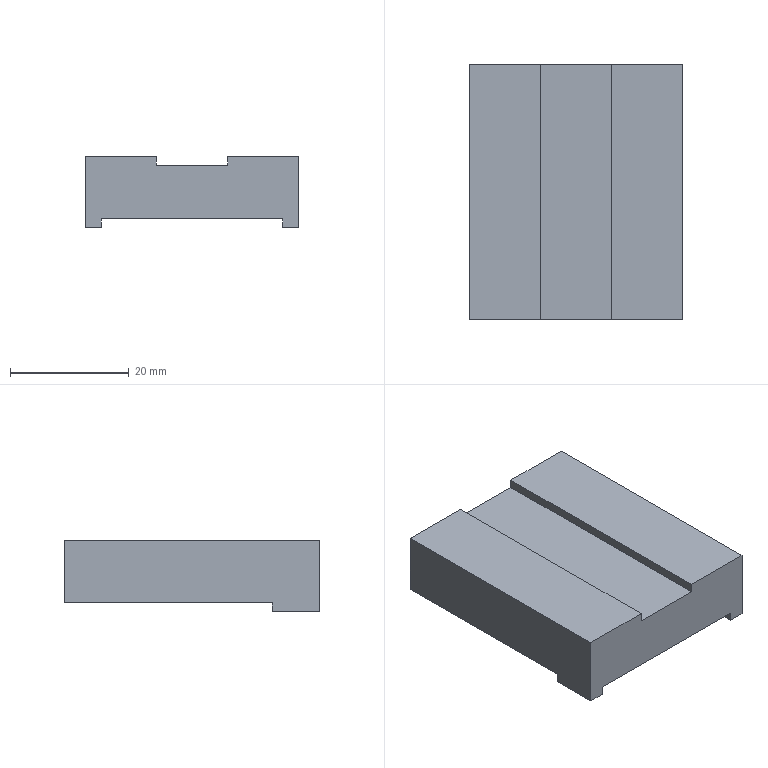Part | SolidWorks | features ICE 3, Extrusion 1 | 1 solid | 16 faces | box 36 x 43 x 12 mm | volume 15546 mm3 | plane 16
STEP:
#1=CARTESIAN_POINT('',(18.,-13.5,-6.));
#2=VERTEX_POINT('',#1);
#3=CARTESIAN_POINT('',(15.25,-13.5,-6.));
#4=VERTEX_POINT('',#3);
#5=CARTESIAN_POINT('',(-18.,-13.5,-6.));
#6=DIRECTION('',(-1.,0.,0.));
#7=VECTOR('',#6,1000.);
#8=LINE('',#5,#7);
#9=EDGE_CURVE('',#2,#4,#8,.T.);
#10=ORIENTED_EDGE('',*,*,#9,.F.);
#11=CARTESIAN_POINT('',(18.,-21.5,-6.));
#12=VERTEX_POINT('',#11);
#13=CARTESIAN_POINT('',(18.,-21.5,-6.));
#14=DIRECTION('',(0.,1.,0.));
#15=VECTOR('',#14,1000.);
#16=LINE('',#13,#15);
#17=EDGE_CURVE('',#12,#2,#16,.T.);
#18=ORIENTED_EDGE('',*,*,#17,.F.);
#19=CARTESIAN_POINT('',(15.25,-21.5,-6.));
#20=VERTEX_POINT('',#19);
#21=CARTESIAN_POINT('',(-18.,-21.5,-6.));
#22=DIRECTION('',(1.,0.,0.));
#23=VECTOR('',#22,1000.);
#24=LINE('',#21,#23);
#25=EDGE_CURVE('',#20,#12,#24,.T.);
#26=ORIENTED_EDGE('',*,*,#25,.F.);
#27=CARTESIAN_POINT('',(15.25,21.5,-6.));
#28=DIRECTION('',(0.,-1.,0.));
#29=VECTOR('',#28,1000.);
#30=LINE('',#27,#29);
#31=EDGE_CURVE('',#4,#20,#30,.T.);
#32=ORIENTED_EDGE('',*,*,#31,.F.);
#33=EDGE_LOOP('',(#10,#18,#26,#32));
#34=FACE_OUTER_BOUND('',#33,.T.);
#35=CARTESIAN_POINT('',(0.,0.,-6.));
#36=DIRECTION('',(0.,0.,-1.));
#37=DIRECTION('',(-1.,0.,0.));
#38=AXIS2_PLACEMENT_3D('',#35,#36,#37);
#39=PLANE('',#38);
#40=ADVANCED_FACE('',(#34),#39,.T.);
#41=CARTESIAN_POINT('',(18.,21.5,6.));
#42=VERTEX_POINT('',#41);
#43=CARTESIAN_POINT('',(6.,21.5,6.));
#44=VERTEX_POINT('',#43);
#45=CARTESIAN_POINT('',(-18.,21.5,6.));
#46=DIRECTION('',(-1.,0.,0.));
#47=VECTOR('',#46,1000.);
#48=LINE('',#45,#47);
#49=EDGE_CURVE('',#42,#44,#48,.T.);
#50=ORIENTED_EDGE('',*,*,#49,.T.);
#51=CARTESIAN_POINT('',(6.,-21.5,6.));
#52=VERTEX_POINT('',#51);
#53=CARTESIAN_POINT('',(6.,21.5,6.));
#54=DIRECTION('',(0.,1.,0.));
#55=VECTOR('',#54,1000.);
#56=LINE('',#53,#55);
#57=EDGE_CURVE('',#52,#44,#56,.T.);
#58=ORIENTED_EDGE('',*,*,#57,.F.);
#59=CARTESIAN_POINT('',(18.,-21.5,6.));
#60=VERTEX_POINT('',#59);
#61=CARTESIAN_POINT('',(-18.,-21.5,6.));
#62=DIRECTION('',(1.,0.,0.));
#63=VECTOR('',#62,1000.);
#64=LINE('',#61,#63);
#65=EDGE_CURVE('',#52,#60,#64,.T.);
#66=ORIENTED_EDGE('',*,*,#65,.T.);
#67=CARTESIAN_POINT('',(18.,-21.5,6.));
#68=DIRECTION('',(0.,1.,0.));
#69=VECTOR('',#68,1000.);
#70=LINE('',#67,#69);
#71=EDGE_CURVE('',#60,#42,#70,.T.);
#72=ORIENTED_EDGE('',*,*,#71,.T.);
#73=EDGE_LOOP('',(#50,#58,#66,#72));
#74=FACE_OUTER_BOUND('',#73,.T.);
#75=CARTESIAN_POINT('',(0.,0.,6.));
#76=DIRECTION('',(0.,0.,-1.));
#77=DIRECTION('',(-1.,0.,0.));
#78=AXIS2_PLACEMENT_3D('',#75,#76,#77);
#79=PLANE('',#78);
#80=ADVANCED_FACE('',(#74),#79,.F.);
#81=ORIENTED_EDGE('',*,*,#17,.T.);
#82=CARTESIAN_POINT('',(18.,-13.5,-4.5));
#83=VERTEX_POINT('',#82);
#84=CARTESIAN_POINT('',(18.,-13.5,-4.5));
#85=DIRECTION('',(0.,0.,-1.));
#86=VECTOR('',#85,1000.);
#87=LINE('',#84,#86);
#88=EDGE_CURVE('',#83,#2,#87,.T.);
#89=ORIENTED_EDGE('',*,*,#88,.F.);
#90=CARTESIAN_POINT('',(18.,21.5,-4.5));
#91=VERTEX_POINT('',#90);
#92=CARTESIAN_POINT('',(18.,21.5,-4.5));
#93=DIRECTION('',(0.,-1.,0.));
#94=VECTOR('',#93,1000.);
#95=LINE('',#92,#94);
#96=EDGE_CURVE('',#91,#83,#95,.T.);
#97=ORIENTED_EDGE('',*,*,#96,.F.);
#98=CARTESIAN_POINT('',(18.,21.5,6.));
#99=DIRECTION('',(0.,0.,-1.));
#100=VECTOR('',#99,1000.);
#101=LINE('',#98,#100);
#102=EDGE_CURVE('',#42,#91,#101,.T.);
#103=ORIENTED_EDGE('',*,*,#102,.F.);
#104=ORIENTED_EDGE('',*,*,#71,.F.);
#105=CARTESIAN_POINT('',(18.,-21.5,6.));
#106=DIRECTION('',(0.,0.,-1.));
#107=VECTOR('',#106,1000.);
#108=LINE('',#105,#107);
#109=EDGE_CURVE('',#60,#12,#108,.T.);
#110=ORIENTED_EDGE('',*,*,#109,.T.);
#111=EDGE_LOOP('',(#81,#89,#97,#103,#104,#110));
#112=FACE_OUTER_BOUND('',#111,.T.);
#113=CARTESIAN_POINT('',(18.,-21.5,6.));
#114=DIRECTION('',(-1.,0.,0.));
#115=DIRECTION('',(0.,0.,1.));
#116=AXIS2_PLACEMENT_3D('',#113,#114,#115);
#117=PLANE('',#116);
#118=ADVANCED_FACE('',(#112),#117,.F.);
#119=ORIENTED_EDGE('',*,*,#102,.T.);
#120=CARTESIAN_POINT('',(-18.,21.5,-4.5));
#121=VERTEX_POINT('',#120);
#122=CARTESIAN_POINT('',(-15.25,21.5,-4.5));
#123=DIRECTION('',(1.,0.,0.));
#124=VECTOR('',#123,1000.);
#125=LINE('',#122,#124);
#126=EDGE_CURVE('',#121,#91,#125,.T.);
#127=ORIENTED_EDGE('',*,*,#126,.F.);
#128=CARTESIAN_POINT('',(-18.,21.5,6.));
#129=VERTEX_POINT('',#128);
#130=CARTESIAN_POINT('',(-18.,21.5,6.));
#131=DIRECTION('',(0.,0.,-1.));
#132=VECTOR('',#131,1000.);
#133=LINE('',#130,#132);
#134=EDGE_CURVE('',#129,#121,#133,.T.);
#135=ORIENTED_EDGE('',*,*,#134,.F.);
#136=CARTESIAN_POINT('',(-6.,21.5,6.));
#137=VERTEX_POINT('',#136);
#138=CARTESIAN_POINT('',(-18.,21.5,6.));
#139=DIRECTION('',(-1.,0.,0.));
#140=VECTOR('',#139,1000.);
#141=LINE('',#138,#140);
#142=EDGE_CURVE('',#137,#129,#141,.T.);
#143=ORIENTED_EDGE('',*,*,#142,.F.);
#144=CARTESIAN_POINT('',(-6.,21.5,4.5));
#145=VERTEX_POINT('',#144);
#146=CARTESIAN_POINT('',(-6.,21.5,4.5));
#147=DIRECTION('',(0.,0.,1.));
#148=VECTOR('',#147,1000.);
#149=LINE('',#146,#148);
#150=EDGE_CURVE('',#145,#137,#149,.T.);
#151=ORIENTED_EDGE('',*,*,#150,.F.);
#152=CARTESIAN_POINT('',(6.,21.5,4.5));
#153=VERTEX_POINT('',#152);
#154=CARTESIAN_POINT('',(6.,21.5,4.5));
#155=DIRECTION('',(-1.,0.,0.));
#156=VECTOR('',#155,1000.);
#157=LINE('',#154,#156);
#158=EDGE_CURVE('',#153,#145,#157,.T.);
#159=ORIENTED_EDGE('',*,*,#158,.F.);
#160=CARTESIAN_POINT('',(6.,21.5,4.5));
#161=DIRECTION('',(0.,0.,1.));
#162=VECTOR('',#161,1000.);
#163=LINE('',#160,#162);
#164=EDGE_CURVE('',#153,#44,#163,.T.);
#165=ORIENTED_EDGE('',*,*,#164,.T.);
#166=ORIENTED_EDGE('',*,*,#49,.F.);
#167=EDGE_LOOP('',(#119,#127,#135,#143,#151,#159,#165,#166));
#168=FACE_OUTER_BOUND('',#167,.T.);
#169=CARTESIAN_POINT('',(-18.,21.5,6.));
#170=DIRECTION('',(0.,-1.,0.));
#171=DIRECTION('',(0.,0.,-1.));
#172=AXIS2_PLACEMENT_3D('',#169,#170,#171);
#173=PLANE('',#172);
#174=ADVANCED_FACE('',(#168),#173,.F.);
#175=CARTESIAN_POINT('',(-18.,-13.5,-4.5));
#176=VERTEX_POINT('',#175);
#177=CARTESIAN_POINT('',(-18.,21.5,-4.5));
#178=DIRECTION('',(0.,1.,0.));
#179=VECTOR('',#178,1000.);
#180=LINE('',#177,#179);
#181=EDGE_CURVE('',#176,#121,#180,.T.);
#182=ORIENTED_EDGE('',*,*,#181,.F.);
#183=CARTESIAN_POINT('',(-18.,-13.5,-6.));
#184=VERTEX_POINT('',#183);
#185=CARTESIAN_POINT('',(-18.,-13.5,-4.5));
#186=DIRECTION('',(0.,0.,-1.));
#187=VECTOR('',#186,1000.);
#188=LINE('',#185,#187);
#189=EDGE_CURVE('',#176,#184,#188,.T.);
#190=ORIENTED_EDGE('',*,*,#189,.T.);
#191=CARTESIAN_POINT('',(-18.,-21.5,-6.));
#192=VERTEX_POINT('',#191);
#193=CARTESIAN_POINT('',(-18.,-21.5,-6.));
#194=DIRECTION('',(0.,-1.,0.));
#195=VECTOR('',#194,1000.);
#196=LINE('',#193,#195);
#197=EDGE_CURVE('',#184,#192,#196,.T.);
#198=ORIENTED_EDGE('',*,*,#197,.T.);
#199=CARTESIAN_POINT('',(-18.,-21.5,6.));
#200=VERTEX_POINT('',#199);
#201=CARTESIAN_POINT('',(-18.,-21.5,6.));
#202=DIRECTION('',(0.,0.,-1.));
#203=VECTOR('',#202,1000.);
#204=LINE('',#201,#203);
#205=EDGE_CURVE('',#200,#192,#204,.T.);
#206=ORIENTED_EDGE('',*,*,#205,.F.);
#207=CARTESIAN_POINT('',(-18.,-21.5,6.));
#208=DIRECTION('',(0.,-1.,0.));
#209=VECTOR('',#208,1000.);
#210=LINE('',#207,#209);
#211=EDGE_CURVE('',#129,#200,#210,.T.);
#212=ORIENTED_EDGE('',*,*,#211,.F.);
#213=ORIENTED_EDGE('',*,*,#134,.T.);
#214=EDGE_LOOP('',(#182,#190,#198,#206,#212,#213));
#215=FACE_OUTER_BOUND('',#214,.T.);
#216=CARTESIAN_POINT('',(-18.,-21.5,6.));
#217=DIRECTION('',(1.,0.,0.));
#218=DIRECTION('',(0.,0.,-1.));
#219=AXIS2_PLACEMENT_3D('',#216,#217,#218);
#220=PLANE('',#219);
#221=ADVANCED_FACE('',(#215),#220,.F.);
#222=CARTESIAN_POINT('',(15.25,-21.5,-4.5));
#223=VERTEX_POINT('',#222);
#224=CARTESIAN_POINT('',(-15.25,-21.5,-4.5));
#225=VERTEX_POINT('',#224);
#226=CARTESIAN_POINT('',(-15.25,-21.5,-4.5));
#227=DIRECTION('',(-1.,0.,0.));
#228=VECTOR('',#227,1000.);
#229=LINE('',#226,#228);
#230=EDGE_CURVE('',#223,#225,#229,.T.);
#231=ORIENTED_EDGE('',*,*,#230,.F.);
#232=CARTESIAN_POINT('',(15.25,-21.5,-4.5));
#233=DIRECTION('',(0.,0.,-1.));
#234=VECTOR('',#233,1000.);
#235=LINE('',#232,#234);
#236=EDGE_CURVE('',#223,#20,#235,.T.);
#237=ORIENTED_EDGE('',*,*,#236,.T.);
#238=ORIENTED_EDGE('',*,*,#25,.T.);
#239=ORIENTED_EDGE('',*,*,#109,.F.);
#240=ORIENTED_EDGE('',*,*,#65,.F.);
#241=CARTESIAN_POINT('',(6.,-21.5,4.5));
#242=VERTEX_POINT('',#241);
#243=CARTESIAN_POINT('',(6.,-21.5,4.5));
#244=DIRECTION('',(0.,0.,1.));
#245=VECTOR('',#244,1000.);
#246=LINE('',#243,#245);
#247=EDGE_CURVE('',#242,#52,#246,.T.);
#248=ORIENTED_EDGE('',*,*,#247,.F.);
#249=CARTESIAN_POINT('',(-6.,-21.5,4.5));
#250=VERTEX_POINT('',#249);
#251=CARTESIAN_POINT('',(6.,-21.5,4.5));
#252=DIRECTION('',(1.,0.,0.));
#253=VECTOR('',#252,1000.);
#254=LINE('',#251,#253);
#255=EDGE_CURVE('',#250,#242,#254,.T.);
#256=ORIENTED_EDGE('',*,*,#255,.F.);
#257=CARTESIAN_POINT('',(-6.,-21.5,6.));
#258=VERTEX_POINT('',#257);
#259=CARTESIAN_POINT('',(-6.,-21.5,4.5));
#260=DIRECTION('',(0.,0.,1.));
#261=VECTOR('',#260,1000.);
#262=LINE('',#259,#261);
#263=EDGE_CURVE('',#250,#258,#262,.T.);
#264=ORIENTED_EDGE('',*,*,#263,.T.);
#265=CARTESIAN_POINT('',(-18.,-21.5,6.));
#266=DIRECTION('',(1.,0.,0.));
#267=VECTOR('',#266,1000.);
#268=LINE('',#265,#267);
#269=EDGE_CURVE('',#200,#258,#268,.T.);
#270=ORIENTED_EDGE('',*,*,#269,.F.);
#271=ORIENTED_EDGE('',*,*,#205,.T.);
#272=CARTESIAN_POINT('',(-15.25,-21.5,-6.));
#273=VERTEX_POINT('',#272);
#274=CARTESIAN_POINT('',(-18.,-21.5,-6.));
#275=DIRECTION('',(1.,0.,0.));
#276=VECTOR('',#275,1000.);
#277=LINE('',#274,#276);
#278=EDGE_CURVE('',#192,#273,#277,.T.);
#279=ORIENTED_EDGE('',*,*,#278,.T.);
#280=CARTESIAN_POINT('',(-15.25,-21.5,-4.5));
#281=DIRECTION('',(0.,0.,-1.));
#282=VECTOR('',#281,1000.);
#283=LINE('',#280,#282);
#284=EDGE_CURVE('',#225,#273,#283,.T.);
#285=ORIENTED_EDGE('',*,*,#284,.F.);
#286=EDGE_LOOP('',(#231,#237,#238,#239,#240,#248,#256,#264,#270,#271,#279,#285));
#287=FACE_OUTER_BOUND('',#286,.T.);
#288=CARTESIAN_POINT('',(-18.,-21.5,6.));
#289=DIRECTION('',(0.,1.,0.));
#290=DIRECTION('',(0.,0.,1.));
#291=AXIS2_PLACEMENT_3D('',#288,#289,#290);
#292=PLANE('',#291);
#293=ADVANCED_FACE('',(#287),#292,.F.);
#294=ORIENTED_EDGE('',*,*,#269,.T.);
#295=CARTESIAN_POINT('',(-6.,21.5,6.));
#296=DIRECTION('',(0.,-1.,0.));
#297=VECTOR('',#296,1000.);
#298=LINE('',#295,#297);
#299=EDGE_CURVE('',#137,#258,#298,.T.);
#300=ORIENTED_EDGE('',*,*,#299,.F.);
#301=ORIENTED_EDGE('',*,*,#142,.T.);
#302=ORIENTED_EDGE('',*,*,#211,.T.);
#303=EDGE_LOOP('',(#294,#300,#301,#302));
#304=FACE_OUTER_BOUND('',#303,.T.);
#305=CARTESIAN_POINT('',(0.,0.,6.));
#306=DIRECTION('',(0.,0.,-1.));
#307=DIRECTION('',(-1.,0.,0.));
#308=AXIS2_PLACEMENT_3D('',#305,#306,#307);
#309=PLANE('',#308);
#310=ADVANCED_FACE('',(#304),#309,.F.);
#311=CARTESIAN_POINT('',(-15.25,-13.5,-6.));
#312=VERTEX_POINT('',#311);
#313=CARTESIAN_POINT('',(-18.,-13.5,-6.));
#314=DIRECTION('',(-1.,0.,0.));
#315=VECTOR('',#314,1000.);
#316=LINE('',#313,#315);
#317=EDGE_CURVE('',#312,#184,#316,.T.);
#318=ORIENTED_EDGE('',*,*,#317,.F.);
#319=CARTESIAN_POINT('',(-15.25,21.5,-6.));
#320=DIRECTION('',(0.,1.,0.));
#321=VECTOR('',#320,1000.);
#322=LINE('',#319,#321);
#323=EDGE_CURVE('',#273,#312,#322,.T.);
#324=ORIENTED_EDGE('',*,*,#323,.F.);
#325=ORIENTED_EDGE('',*,*,#278,.F.);
#326=ORIENTED_EDGE('',*,*,#197,.F.);
#327=EDGE_LOOP('',(#318,#324,#325,#326));
#328=FACE_OUTER_BOUND('',#327,.T.);
#329=CARTESIAN_POINT('',(0.,0.,-6.));
#330=DIRECTION('',(0.,0.,-1.));
#331=DIRECTION('',(-1.,0.,0.));
#332=AXIS2_PLACEMENT_3D('',#329,#330,#331);
#333=PLANE('',#332);
#334=ADVANCED_FACE('',(#328),#333,.T.);
#335=ORIENTED_EDGE('',*,*,#57,.T.);
#336=ORIENTED_EDGE('',*,*,#164,.F.);
#337=CARTESIAN_POINT('',(6.,21.5,4.5));
#338=DIRECTION('',(0.,1.,0.));
#339=VECTOR('',#338,1000.);
#340=LINE('',#337,#339);
#341=EDGE_CURVE('',#242,#153,#340,.T.);
#342=ORIENTED_EDGE('',*,*,#341,.F.);
#343=ORIENTED_EDGE('',*,*,#247,.T.);
#344=EDGE_LOOP('',(#335,#336,#342,#343));
#345=FACE_OUTER_BOUND('',#344,.T.);
#346=CARTESIAN_POINT('',(6.,21.5,4.5));
#347=DIRECTION('',(1.,0.,0.));
#348=DIRECTION('',(0.,1.,0.));
#349=AXIS2_PLACEMENT_3D('',#346,#347,#348);
#350=PLANE('',#349);
#351=ADVANCED_FACE('',(#345),#350,.F.);
#352=ORIENTED_EDGE('',*,*,#299,.T.);
#353=ORIENTED_EDGE('',*,*,#263,.F.);
#354=CARTESIAN_POINT('',(-6.,21.5,4.5));
#355=DIRECTION('',(0.,-1.,0.));
#356=VECTOR('',#355,1000.);
#357=LINE('',#354,#356);
#358=EDGE_CURVE('',#145,#250,#357,.T.);
#359=ORIENTED_EDGE('',*,*,#358,.F.);
#360=ORIENTED_EDGE('',*,*,#150,.T.);
#361=EDGE_LOOP('',(#352,#353,#359,#360));
#362=FACE_OUTER_BOUND('',#361,.T.);
#363=CARTESIAN_POINT('',(-6.,21.5,4.5));
#364=DIRECTION('',(-1.,0.,0.));
#365=DIRECTION('',(0.,-1.,0.));
#366=AXIS2_PLACEMENT_3D('',#363,#364,#365);
#367=PLANE('',#366);
#368=ADVANCED_FACE('',(#362),#367,.F.);
#369=ORIENTED_EDGE('',*,*,#341,.T.);
#370=ORIENTED_EDGE('',*,*,#158,.T.);
#371=ORIENTED_EDGE('',*,*,#358,.T.);
#372=ORIENTED_EDGE('',*,*,#255,.T.);
#373=EDGE_LOOP('',(#369,#370,#371,#372));
#374=FACE_OUTER_BOUND('',#373,.T.);
#375=CARTESIAN_POINT('',(0.,0.,4.5));
#376=DIRECTION('',(0.,0.,-1.));
#377=DIRECTION('',(-1.,0.,0.));
#378=AXIS2_PLACEMENT_3D('',#375,#376,#377);
#379=PLANE('',#378);
#380=ADVANCED_FACE('',(#374),#379,.F.);
#381=CARTESIAN_POINT('',(15.25,-13.5,-4.5));
#382=VERTEX_POINT('',#381);
#383=CARTESIAN_POINT('',(15.25,21.5,-4.5));
#384=DIRECTION('',(0.,-1.,0.));
#385=VECTOR('',#384,1000.);
#386=LINE('',#383,#385);
#387=EDGE_CURVE('',#382,#223,#386,.T.);
#388=ORIENTED_EDGE('',*,*,#387,.F.);
#389=CARTESIAN_POINT('',(15.25,-13.5,-4.5));
#390=DIRECTION('',(0.,0.,-1.));
#391=VECTOR('',#390,1000.);
#392=LINE('',#389,#391);
#393=EDGE_CURVE('',#382,#4,#392,.T.);
#394=ORIENTED_EDGE('',*,*,#393,.T.);
#395=ORIENTED_EDGE('',*,*,#31,.T.);
#396=ORIENTED_EDGE('',*,*,#236,.F.);
#397=EDGE_LOOP('',(#388,#394,#395,#396));
#398=FACE_OUTER_BOUND('',#397,.T.);
#399=CARTESIAN_POINT('',(15.25,21.5,-4.5));
#400=DIRECTION('',(1.,0.,0.));
#401=DIRECTION('',(0.,0.,-1.));
#402=AXIS2_PLACEMENT_3D('',#399,#400,#401);
#403=PLANE('',#402);
#404=ADVANCED_FACE('',(#398),#403,.F.);
#405=ORIENTED_EDGE('',*,*,#323,.T.);
#406=CARTESIAN_POINT('',(-15.25,-13.5,-4.5));
#407=VERTEX_POINT('',#406);
#408=CARTESIAN_POINT('',(-15.25,-13.5,-4.5));
#409=DIRECTION('',(0.,0.,1.));
#410=VECTOR('',#409,1000.);
#411=LINE('',#408,#410);
#412=EDGE_CURVE('',#312,#407,#411,.T.);
#413=ORIENTED_EDGE('',*,*,#412,.T.);
#414=CARTESIAN_POINT('',(-15.25,21.5,-4.5));
#415=DIRECTION('',(0.,1.,0.));
#416=VECTOR('',#415,1000.);
#417=LINE('',#414,#416);
#418=EDGE_CURVE('',#225,#407,#417,.T.);
#419=ORIENTED_EDGE('',*,*,#418,.F.);
#420=ORIENTED_EDGE('',*,*,#284,.T.);
#421=EDGE_LOOP('',(#405,#413,#419,#420));
#422=FACE_OUTER_BOUND('',#421,.T.);
#423=CARTESIAN_POINT('',(-15.25,21.5,-4.5));
#424=DIRECTION('',(-1.,0.,0.));
#425=DIRECTION('',(0.,0.,1.));
#426=AXIS2_PLACEMENT_3D('',#423,#424,#425);
#427=PLANE('',#426);
#428=ADVANCED_FACE('',(#422),#427,.F.);
#429=ORIENTED_EDGE('',*,*,#418,.T.);
#430=CARTESIAN_POINT('',(-18.,-13.5,-4.5));
#431=DIRECTION('',(-1.,0.,0.));
#432=VECTOR('',#431,1000.);
#433=LINE('',#430,#432);
#434=EDGE_CURVE('',#407,#176,#433,.T.);
#435=ORIENTED_EDGE('',*,*,#434,.T.);
#436=ORIENTED_EDGE('',*,*,#181,.T.);
#437=ORIENTED_EDGE('',*,*,#126,.T.);
#438=ORIENTED_EDGE('',*,*,#96,.T.);
#439=CARTESIAN_POINT('',(-18.,-13.5,-4.5));
#440=DIRECTION('',(-1.,0.,0.));
#441=VECTOR('',#440,1000.);
#442=LINE('',#439,#441);
#443=EDGE_CURVE('',#83,#382,#442,.T.);
#444=ORIENTED_EDGE('',*,*,#443,.T.);
#445=ORIENTED_EDGE('',*,*,#387,.T.);
#446=ORIENTED_EDGE('',*,*,#230,.T.);
#447=EDGE_LOOP('',(#429,#435,#436,#437,#438,#444,#445,#446));
#448=FACE_OUTER_BOUND('',#447,.T.);
#449=CARTESIAN_POINT('',(0.,0.,-4.5));
#450=DIRECTION('',(0.,0.,1.));
#451=DIRECTION('',(1.,0.,0.));
#452=AXIS2_PLACEMENT_3D('',#449,#450,#451);
#453=PLANE('',#452);
#454=ADVANCED_FACE('',(#448),#453,.F.);
#455=ORIENTED_EDGE('',*,*,#317,.T.);
#456=ORIENTED_EDGE('',*,*,#189,.F.);
#457=ORIENTED_EDGE('',*,*,#434,.F.);
#458=ORIENTED_EDGE('',*,*,#412,.F.);
#459=EDGE_LOOP('',(#455,#456,#457,#458));
#460=FACE_OUTER_BOUND('',#459,.T.);
#461=CARTESIAN_POINT('',(-18.,-13.5,-4.5));
#462=DIRECTION('',(0.,-1.,0.));
#463=DIRECTION('',(1.,0.,0.));
#464=AXIS2_PLACEMENT_3D('',#461,#462,#463);
#465=PLANE('',#464);
#466=ADVANCED_FACE('',(#460),#465,.F.);
#467=ORIENTED_EDGE('',*,*,#443,.F.);
#468=ORIENTED_EDGE('',*,*,#88,.T.);
#469=ORIENTED_EDGE('',*,*,#9,.T.);
#470=ORIENTED_EDGE('',*,*,#393,.F.);
#471=EDGE_LOOP('',(#467,#468,#469,#470));
#472=FACE_OUTER_BOUND('',#471,.T.);
#473=CARTESIAN_POINT('',(-18.,-13.5,-4.5));
#474=DIRECTION('',(0.,-1.,0.));
#475=DIRECTION('',(1.,0.,0.));
#476=AXIS2_PLACEMENT_3D('',#473,#474,#475);
#477=PLANE('',#476);
#478=ADVANCED_FACE('',(#472),#477,.F.);
#479=CLOSED_SHELL('',(#40,#80,#118,#174,#221,#293,#310,#334,#351,#368,#380,#404,#428,#454,#466,#478));
#480=MANIFOLD_SOLID_BREP('',#479);
#481=CARTESIAN_POINT('',(0.,0.,0.));
#482=DIRECTION('',(0.,0.,1.));
#483=DIRECTION('',(1.,0.,0.));
#484=AXIS2_PLACEMENT_3D('',#481,#482,#483);
#485=(LENGTH_UNIT()NAMED_UNIT(*)SI_UNIT(.MILLI.,.METRE.));
#486=UNCERTAINTY_MEASURE_WITH_UNIT(LENGTH_MEASURE(0.00001),#485,'','');
#487=(NAMED_UNIT(*)PLANE_ANGLE_UNIT()SI_UNIT($,.RADIAN.));
#488=(NAMED_UNIT(*)SI_UNIT($,.STERADIAN.)SOLID_ANGLE_UNIT());
#489=(GEOMETRIC_REPRESENTATION_CONTEXT(3)GLOBAL_UNCERTAINTY_ASSIGNED_CONTEXT((#486))GLOBAL_UNIT_ASSIGNED_CONTEXT((#485,#487,#488))REPRESENTATION_CONTEXT('',''));
#490=ADVANCED_BREP_SHAPE_REPRESENTATION('',(#480,#484),#489);